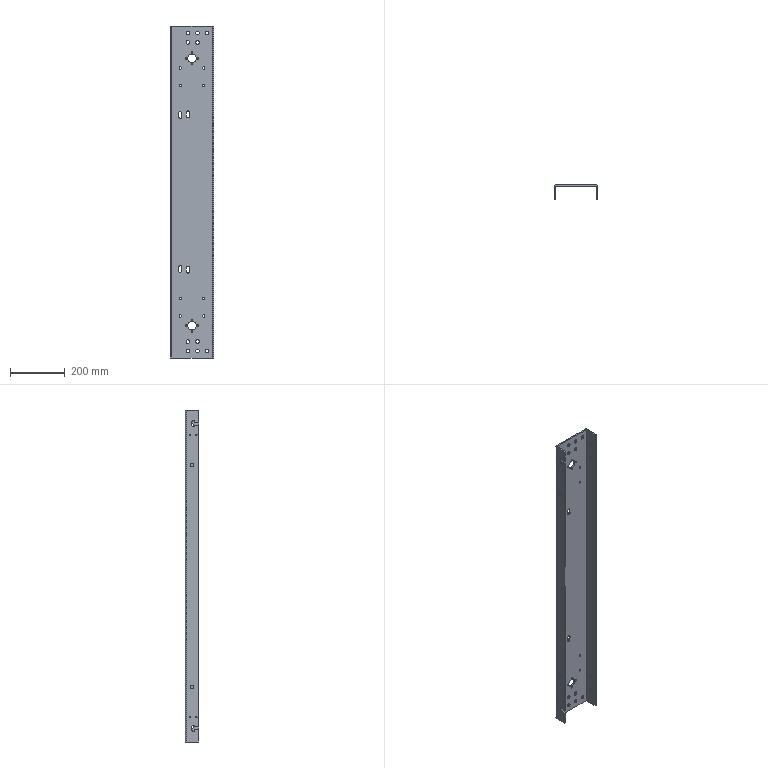Part | 1 solid | 130 faces | box 160 x 50 x 1210 mm | volume 1463171 mm3 | cylinder 96 | plane 34 | commonest cylinder face diameters 13 x32 6 x16 8.5 x16 12 x14 5 x8 11 x4